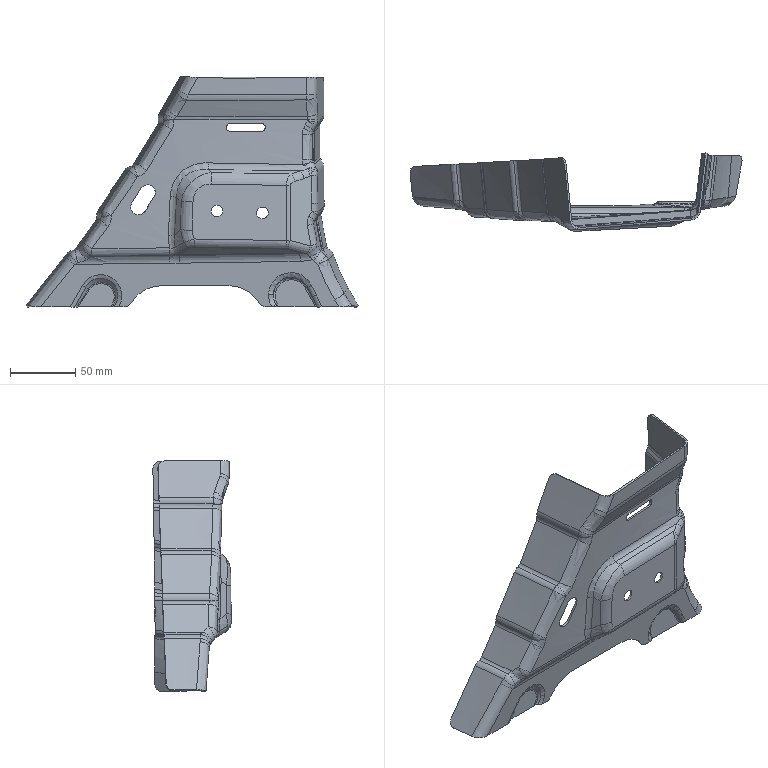Part | STEP file | FNA5401671 | 1 solid | 406 faces | box 254.233 x 59.892 x 176.91 mm | volume 64853 mm3 | spline 330 | cylinder 46 | other 13 | sphere 12 | plane 5 | commonest cylinder face diameters 9 x11 12 x10 15 x6 6 x5 20 x3 3 x2